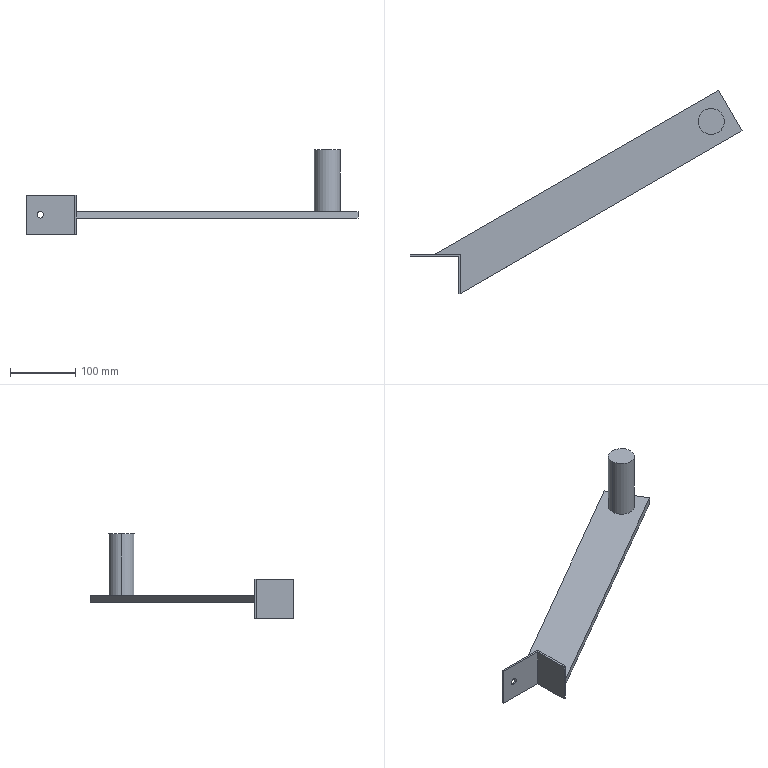Part | STEP file | 1 solid | 19 faces | box 510.013 x 312.321 x 130 mm | volume 492742 mm3 | plane 15 | cylinder 4 | commonest cylinder face diameters 10 x2 40 x2
STEP:
#1=CARTESIAN_POINT('',(0.,0.,0.));
#2=DIRECTION('',(0.,0.,1.));
#3=DIRECTION('',(1.,0.,0.));
#4=AXIS2_PLACEMENT_3D('',#1,#2,#3);
#5=CARTESIAN_POINT('',(-3.745,29.61,-5.));
#6=VERTEX_POINT('',#5);
#7=CARTESIAN_POINT('',(-3.745,26.61,-5.));
#8=VERTEX_POINT('',#7);
#9=CARTESIAN_POINT('',(-3.745,29.61,-5.));
#10=DIRECTION('',(0.,-1.,0.));
#11=VECTOR('',#10,1.);
#12=LINE('',#9,#11);
#13=CARTESIAN_POINT('',(-3.745,29.61,0.));
#14=DIRECTION('',(0.,-1.,0.));
#15=DIRECTION('',(0.,0.,-1.));
#16=AXIS2_PLACEMENT_3D('',#13,#14,#15);
#17=CYLINDRICAL_SURFACE('',#16,5.);
#18=CARTESIAN_POINT('',(6.283,0.));
#19=DIRECTION('',(0.,1.));
#20=VECTOR('',#19,1.);
#21=LINE('',#18,#20);
#22=(GEOMETRIC_REPRESENTATION_CONTEXT(2)PARAMETRIC_REPRESENTATION_CONTEXT()REPRESENTATION_CONTEXT('',''));
#23=DEFINITIONAL_REPRESENTATION('',(#21),#22);
#24=PCURVE('',#17,#23);
#25=CARTESIAN_POINT('',(-3.745,29.61,0.));
#26=DIRECTION('',(0.,-1.,0.));
#27=DIRECTION('',(0.,0.,-1.));
#28=AXIS2_PLACEMENT_3D('',#25,#26,#27);
#29=CYLINDRICAL_SURFACE('',#28,5.);
#30=CARTESIAN_POINT('',(0.,0.));
#31=DIRECTION('',(0.,1.));
#32=VECTOR('',#31,1.);
#33=LINE('',#30,#32);
#34=(GEOMETRIC_REPRESENTATION_CONTEXT(2)PARAMETRIC_REPRESENTATION_CONTEXT()REPRESENTATION_CONTEXT('',''));
#35=DEFINITIONAL_REPRESENTATION('',(#33),#34);
#36=PCURVE('',#29,#35);
#37=SURFACE_CURVE('',#12,(#24,#36),.PCURVE_S1.);
#38=EDGE_CURVE('',#6,#8,#37,.T.);
#39=ORIENTED_EDGE('',*,*,#38,.T.);
#40=CARTESIAN_POINT('',(-3.745,26.61,5.));
#41=VERTEX_POINT('',#40);
#42=CARTESIAN_POINT('',(-3.745,26.61,0.));
#43=DIRECTION('',(0.,1.,0.));
#44=DIRECTION('',(0.,0.,-1.));
#45=AXIS2_PLACEMENT_3D('',#42,#43,#44);
#46=CIRCLE('',#45,5.);
#47=CARTESIAN_POINT('',(6.283,3.));
#48=DIRECTION('',(-1.,0.));
#49=VECTOR('',#48,1.);
#50=LINE('',#47,#49);
#51=(GEOMETRIC_REPRESENTATION_CONTEXT(2)PARAMETRIC_REPRESENTATION_CONTEXT()REPRESENTATION_CONTEXT('',''));
#52=DEFINITIONAL_REPRESENTATION('',(#50),#51);
#53=PCURVE('',#17,#52);
#54=CARTESIAN_POINT('',(-25.745,26.61,0.));
#55=DIRECTION('',(0.,-1.,0.));
#56=DIRECTION('',(1.,0.,0.));
#57=AXIS2_PLACEMENT_3D('',#54,#55,#56);
#58=PLANE('',#57);
#59=CARTESIAN_POINT('',(22.,-5.));
#60=CARTESIAN_POINT('',(13.34,-5.));
#61=CARTESIAN_POINT('',(17.67,2.5));
#62=CARTESIAN_POINT('',(22.,10.));
#63=CARTESIAN_POINT('',(26.33,2.5));
#64=CARTESIAN_POINT('',(30.66,-5.));
#65=CARTESIAN_POINT('',(22.,-5.));
#66=(BOUNDED_CURVE()B_SPLINE_CURVE(2,(#59,#60,#61,#62,#63,#64,#65),.UNSPECIFIED.,.T.,.F.)B_SPLINE_CURVE_WITH_KNOTS((1,2,2,2,2,1),(-2.094,0.,2.094,4.189,6.283,8.378),.UNSPECIFIED.)CURVE()GEOMETRIC_REPRESENTATION_ITEM()RATIONAL_B_SPLINE_CURVE((1.,0.5,1.,0.5,1.,0.5,1.))REPRESENTATION_ITEM(''));
#67=(GEOMETRIC_REPRESENTATION_CONTEXT(2)PARAMETRIC_REPRESENTATION_CONTEXT()REPRESENTATION_CONTEXT('',''));
#68=DEFINITIONAL_REPRESENTATION('',(#66),#67);
#69=PCURVE('',#58,#68);
#70=SURFACE_CURVE('',#46,(#53,#69),.PCURVE_S1.);
#71=EDGE_CURVE('',#8,#41,#70,.T.);
#72=ORIENTED_EDGE('',*,*,#71,.T.);
#73=CARTESIAN_POINT('',(-3.745,29.61,5.));
#74=VERTEX_POINT('',#73);
#75=CARTESIAN_POINT('',(-3.745,29.61,5.));
#76=DIRECTION('',(0.,-1.,0.));
#77=VECTOR('',#76,1.);
#78=LINE('',#75,#77);
#79=CARTESIAN_POINT('',(3.142,0.));
#80=DIRECTION('',(0.,1.));
#81=VECTOR('',#80,1.);
#82=LINE('',#79,#81);
#83=(GEOMETRIC_REPRESENTATION_CONTEXT(2)PARAMETRIC_REPRESENTATION_CONTEXT()REPRESENTATION_CONTEXT('',''));
#84=DEFINITIONAL_REPRESENTATION('',(#82),#83);
#85=PCURVE('',#17,#84);
#86=CARTESIAN_POINT('',(3.142,0.));
#87=DIRECTION('',(0.,1.));
#88=VECTOR('',#87,1.);
#89=LINE('',#86,#88);
#90=(GEOMETRIC_REPRESENTATION_CONTEXT(2)PARAMETRIC_REPRESENTATION_CONTEXT()REPRESENTATION_CONTEXT('',''));
#91=DEFINITIONAL_REPRESENTATION('',(#89),#90);
#92=PCURVE('',#29,#91);
#93=SURFACE_CURVE('',#78,(#85,#92),.PCURVE_S1.);
#94=EDGE_CURVE('',#74,#41,#93,.T.);
#95=ORIENTED_EDGE('',*,*,#94,.F.);
#96=CARTESIAN_POINT('',(-3.745,29.61,0.));
#97=DIRECTION('',(0.,-1.,0.));
#98=DIRECTION('',(0.,0.,-1.));
#99=AXIS2_PLACEMENT_3D('',#96,#97,#98);
#100=CIRCLE('',#99,5.);
#101=CARTESIAN_POINT('',(0.,0.));
#102=DIRECTION('',(1.,0.));
#103=VECTOR('',#102,1.);
#104=LINE('',#101,#103);
#105=(GEOMETRIC_REPRESENTATION_CONTEXT(2)PARAMETRIC_REPRESENTATION_CONTEXT()REPRESENTATION_CONTEXT('',''));
#106=DEFINITIONAL_REPRESENTATION('',(#104),#105);
#107=PCURVE('',#17,#106);
#108=CARTESIAN_POINT('',(51.255,29.61,0.));
#109=DIRECTION('',(0.,1.,0.));
#110=DIRECTION('',(0.,0.,1.));
#111=AXIS2_PLACEMENT_3D('',#108,#109,#110);
#112=PLANE('',#111);
#113=CARTESIAN_POINT('',(-5.,-55.));
#114=CARTESIAN_POINT('',(-5.,-46.34));
#115=CARTESIAN_POINT('',(2.5,-50.67));
#116=CARTESIAN_POINT('',(10.,-55.));
#117=CARTESIAN_POINT('',(2.5,-59.33));
#118=CARTESIAN_POINT('',(-5.,-63.66));
#119=CARTESIAN_POINT('',(-5.,-55.));
#120=(BOUNDED_CURVE()B_SPLINE_CURVE(2,(#113,#114,#115,#116,#117,#118,#119),.UNSPECIFIED.,.T.,.F.)B_SPLINE_CURVE_WITH_KNOTS((1,2,2,2,2,1),(-2.094,0.,2.094,4.189,6.283,8.378),.UNSPECIFIED.)CURVE()GEOMETRIC_REPRESENTATION_ITEM()RATIONAL_B_SPLINE_CURVE((1.,0.5,1.,0.5,1.,0.5,1.))REPRESENTATION_ITEM(''));
#121=(GEOMETRIC_REPRESENTATION_CONTEXT(2)PARAMETRIC_REPRESENTATION_CONTEXT()REPRESENTATION_CONTEXT('',''));
#122=DEFINITIONAL_REPRESENTATION('',(#120),#121);
#123=PCURVE('',#112,#122);
#124=SURFACE_CURVE('',#100,(#107,#123),.PCURVE_S1.);
#125=EDGE_CURVE('',#74,#6,#124,.T.);
#126=ORIENTED_EDGE('',*,*,#125,.T.);
#127=EDGE_LOOP('',(#39,#72,#95,#126));
#128=FACE_BOUND('',#127,.F.);
#129=ADVANCED_FACE('',(#128),#17,.F.);
#130=CARTESIAN_POINT('',(417.097,233.973,5.));
#131=VERTEX_POINT('',#130);
#132=CARTESIAN_POINT('',(457.097,233.973,5.));
#133=VERTEX_POINT('',#132);
#134=CARTESIAN_POINT('',(437.097,233.973,5.));
#135=DIRECTION('',(0.,0.,-1.));
#136=DIRECTION('',(1.,0.,0.));
#137=AXIS2_PLACEMENT_3D('',#134,#135,#136);
#138=CIRCLE('',#137,20.);
#139=CARTESIAN_POINT('',(437.097,233.973,5.));
#140=DIRECTION('',(0.,0.,1.));
#141=DIRECTION('',(1.,0.,0.));
#142=AXIS2_PLACEMENT_3D('',#139,#140,#141);
#143=CYLINDRICAL_SURFACE('',#142,20.);
#144=CARTESIAN_POINT('',(6.283,0.));
#145=DIRECTION('',(-1.,0.));
#146=VECTOR('',#145,1.);
#147=LINE('',#144,#146);
#148=(GEOMETRIC_REPRESENTATION_CONTEXT(2)PARAMETRIC_REPRESENTATION_CONTEXT()REPRESENTATION_CONTEXT('',''));
#149=DEFINITIONAL_REPRESENTATION('',(#147),#148);
#150=PCURVE('',#143,#149);
#151=CARTESIAN_POINT('',(244.528,123.338,5.));
#152=DIRECTION('',(0.,0.,1.));
#153=DIRECTION('',(1.,0.,0.));
#154=AXIS2_PLACEMENT_3D('',#151,#152,#153);
#155=PLANE('',#154);
#156=CARTESIAN_POINT('',(212.569,110.635));
#157=CARTESIAN_POINT('',(212.569,75.994));
#158=CARTESIAN_POINT('',(182.569,93.314));
#159=CARTESIAN_POINT('',(152.569,110.635));
#160=CARTESIAN_POINT('',(182.569,127.955));
#161=CARTESIAN_POINT('',(212.569,145.276));
#162=CARTESIAN_POINT('',(212.569,110.635));
#163=(BOUNDED_CURVE()B_SPLINE_CURVE(2,(#156,#157,#158,#159,#160,#161,#162),.UNSPECIFIED.,.T.,.F.)B_SPLINE_CURVE_WITH_KNOTS((1,2,2,2,2,1),(-2.094,0.,2.094,4.189,6.283,8.378),.UNSPECIFIED.)CURVE()GEOMETRIC_REPRESENTATION_ITEM()RATIONAL_B_SPLINE_CURVE((1.,0.5,1.,0.5,1.,0.5,1.))REPRESENTATION_ITEM(''));
#164=(GEOMETRIC_REPRESENTATION_CONTEXT(2)PARAMETRIC_REPRESENTATION_CONTEXT()REPRESENTATION_CONTEXT('',''));
#165=DEFINITIONAL_REPRESENTATION('',(#163),#164);
#166=PCURVE('',#155,#165);
#167=SURFACE_CURVE('',#138,(#150,#166),.PCURVE_S1.);
#168=EDGE_CURVE('',#131,#133,#167,.T.);
#169=ORIENTED_EDGE('',*,*,#168,.F.);
#170=CARTESIAN_POINT('',(417.097,233.973,100.));
#171=VERTEX_POINT('',#170);
#172=CARTESIAN_POINT('',(417.097,233.973,5.));
#173=DIRECTION('',(0.,0.,1.));
#174=VECTOR('',#173,1.);
#175=LINE('',#172,#174);
#176=CARTESIAN_POINT('',(3.142,0.));
#177=DIRECTION('',(0.,1.));
#178=VECTOR('',#177,1.);
#179=LINE('',#176,#178);
#180=(GEOMETRIC_REPRESENTATION_CONTEXT(2)PARAMETRIC_REPRESENTATION_CONTEXT()REPRESENTATION_CONTEXT('',''));
#181=DEFINITIONAL_REPRESENTATION('',(#179),#180);
#182=PCURVE('',#143,#181);
#183=CARTESIAN_POINT('',(437.097,233.973,5.));
#184=DIRECTION('',(0.,0.,1.));
#185=DIRECTION('',(1.,0.,0.));
#186=AXIS2_PLACEMENT_3D('',#183,#184,#185);
#187=CYLINDRICAL_SURFACE('',#186,20.);
#188=CARTESIAN_POINT('',(3.142,0.));
#189=DIRECTION('',(0.,1.));
#190=VECTOR('',#189,1.);
#191=LINE('',#188,#190);
#192=(GEOMETRIC_REPRESENTATION_CONTEXT(2)PARAMETRIC_REPRESENTATION_CONTEXT()REPRESENTATION_CONTEXT('',''));
#193=DEFINITIONAL_REPRESENTATION('',(#191),#192);
#194=PCURVE('',#187,#193);
#195=SURFACE_CURVE('',#175,(#182,#194),.PCURVE_S1.);
#196=EDGE_CURVE('',#131,#171,#195,.T.);
#197=ORIENTED_EDGE('',*,*,#196,.T.);
#198=CARTESIAN_POINT('',(457.097,233.973,100.));
#199=VERTEX_POINT('',#198);
#200=CARTESIAN_POINT('',(437.097,233.973,100.));
#201=DIRECTION('',(0.,0.,-1.));
#202=DIRECTION('',(1.,0.,0.));
#203=AXIS2_PLACEMENT_3D('',#200,#201,#202);
#204=CIRCLE('',#203,20.);
#205=CARTESIAN_POINT('',(6.283,95.));
#206=DIRECTION('',(-1.,0.));
#207=VECTOR('',#206,1.);
#208=LINE('',#205,#207);
#209=(GEOMETRIC_REPRESENTATION_CONTEXT(2)PARAMETRIC_REPRESENTATION_CONTEXT()REPRESENTATION_CONTEXT('',''));
#210=DEFINITIONAL_REPRESENTATION('',(#208),#209);
#211=PCURVE('',#143,#210);
#212=CARTESIAN_POINT('',(437.097,233.973,100.));
#213=DIRECTION('',(0.,0.,1.));
#214=DIRECTION('',(1.,0.,0.));
#215=AXIS2_PLACEMENT_3D('',#212,#213,#214);
#216=PLANE('',#215);
#217=CARTESIAN_POINT('',(20.,0.));
#218=CARTESIAN_POINT('',(20.,-34.641));
#219=CARTESIAN_POINT('',(-10.,-17.321));
#220=CARTESIAN_POINT('',(-40.,0.));
#221=CARTESIAN_POINT('',(-10.,17.321));
#222=CARTESIAN_POINT('',(20.,34.641));
#223=CARTESIAN_POINT('',(20.,0.));
#224=(BOUNDED_CURVE()B_SPLINE_CURVE(2,(#217,#218,#219,#220,#221,#222,#223),.UNSPECIFIED.,.T.,.F.)B_SPLINE_CURVE_WITH_KNOTS((1,2,2,2,2,1),(-2.094,0.,2.094,4.189,6.283,8.378),.UNSPECIFIED.)CURVE()GEOMETRIC_REPRESENTATION_ITEM()RATIONAL_B_SPLINE_CURVE((1.,0.5,1.,0.5,1.,0.5,1.))REPRESENTATION_ITEM(''));
#225=(GEOMETRIC_REPRESENTATION_CONTEXT(2)PARAMETRIC_REPRESENTATION_CONTEXT()REPRESENTATION_CONTEXT('',''));
#226=DEFINITIONAL_REPRESENTATION('',(#224),#225);
#227=PCURVE('',#216,#226);
#228=SURFACE_CURVE('',#204,(#211,#227),.PCURVE_S1.);
#229=EDGE_CURVE('',#171,#199,#228,.T.);
#230=ORIENTED_EDGE('',*,*,#229,.T.);
#231=CARTESIAN_POINT('',(457.097,233.973,5.));
#232=DIRECTION('',(0.,0.,1.));
#233=VECTOR('',#232,1.);
#234=LINE('',#231,#233);
#235=CARTESIAN_POINT('',(0.,0.));
#236=DIRECTION('',(0.,1.));
#237=VECTOR('',#236,1.);
#238=LINE('',#235,#237);
#239=(GEOMETRIC_REPRESENTATION_CONTEXT(2)PARAMETRIC_REPRESENTATION_CONTEXT()REPRESENTATION_CONTEXT('',''));
#240=DEFINITIONAL_REPRESENTATION('',(#238),#239);
#241=PCURVE('',#143,#240);
#242=CARTESIAN_POINT('',(6.283,0.));
#243=DIRECTION('',(0.,1.));
#244=VECTOR('',#243,1.);
#245=LINE('',#242,#244);
#246=(GEOMETRIC_REPRESENTATION_CONTEXT(2)PARAMETRIC_REPRESENTATION_CONTEXT()REPRESENTATION_CONTEXT('',''));
#247=DEFINITIONAL_REPRESENTATION('',(#245),#246);
#248=PCURVE('',#187,#247);
#249=SURFACE_CURVE('',#234,(#241,#248),.PCURVE_S1.);
#250=EDGE_CURVE('',#133,#199,#249,.T.);
#251=ORIENTED_EDGE('',*,*,#250,.F.);
#252=EDGE_LOOP('',(#169,#197,#230,#251));
#253=FACE_BOUND('',#252,.T.);
#254=ADVANCED_FACE('',(#253),#143,.T.);
#255=CARTESIAN_POINT('',(11.255,29.61,-5.));
#256=VERTEX_POINT('',#255);
#257=CARTESIAN_POINT('',(448.287,281.931,-5.));
#258=VERTEX_POINT('',#257);
#259=CARTESIAN_POINT('',(11.255,29.61,-5.));
#260=DIRECTION('',(0.866,0.5,0.));
#261=VECTOR('',#260,1.);
#262=LINE('',#259,#261);
#263=CARTESIAN_POINT('',(244.528,123.338,-5.));
#264=DIRECTION('',(0.,0.,-1.));
#265=DIRECTION('',(-1.,0.,0.));
#266=AXIS2_PLACEMENT_3D('',#263,#264,#265);
#267=PLANE('',#266);
#268=CARTESIAN_POINT('',(233.273,-93.728));
#269=DIRECTION('',(-0.866,0.5));
#270=VECTOR('',#269,1.);
#271=LINE('',#268,#270);
#272=(GEOMETRIC_REPRESENTATION_CONTEXT(2)PARAMETRIC_REPRESENTATION_CONTEXT()REPRESENTATION_CONTEXT('',''));
#273=DEFINITIONAL_REPRESENTATION('',(#271),#272);
#274=PCURVE('',#267,#273);
#275=CARTESIAN_POINT('',(448.287,281.931,0.));
#276=DIRECTION('',(-0.5,0.866,0.));
#277=DIRECTION('',(-0.866,-0.5,0.));
#278=AXIS2_PLACEMENT_3D('',#275,#276,#277);
#279=PLANE('',#278);
#280=CARTESIAN_POINT('',(504.641,-5.));
#281=DIRECTION('',(-1.,0.));
#282=VECTOR('',#281,1.);
#283=LINE('',#280,#282);
#284=(GEOMETRIC_REPRESENTATION_CONTEXT(2)PARAMETRIC_REPRESENTATION_CONTEXT()REPRESENTATION_CONTEXT('',''));
#285=DEFINITIONAL_REPRESENTATION('',(#283),#284);
#286=PCURVE('',#279,#285);
#287=SURFACE_CURVE('',#262,(#274,#286),.PCURVE_S1.);
#288=EDGE_CURVE('',#256,#258,#287,.T.);
#289=ORIENTED_EDGE('',*,*,#288,.T.);
#290=CARTESIAN_POINT('',(484.268,219.61,-5.));
#291=VERTEX_POINT('',#290);
#292=CARTESIAN_POINT('',(448.287,281.931,-5.));
#293=DIRECTION('',(0.5,-0.866,0.));
#294=VECTOR('',#293,1.);
#295=LINE('',#292,#294);
#296=CARTESIAN_POINT('',(-203.759,158.592));
#297=DIRECTION('',(-0.5,-0.866));
#298=VECTOR('',#297,1.);
#299=LINE('',#296,#298);
#300=(GEOMETRIC_REPRESENTATION_CONTEXT(2)PARAMETRIC_REPRESENTATION_CONTEXT()REPRESENTATION_CONTEXT('',''));
#301=DEFINITIONAL_REPRESENTATION('',(#299),#300);
#302=PCURVE('',#267,#301);
#303=CARTESIAN_POINT('',(484.268,219.61,0.));
#304=DIRECTION('',(0.866,0.5,0.));
#305=DIRECTION('',(-0.5,0.866,0.));
#306=AXIS2_PLACEMENT_3D('',#303,#304,#305);
#307=PLANE('',#306);
#308=CARTESIAN_POINT('',(71.962,-5.));
#309=DIRECTION('',(-1.,0.));
#310=VECTOR('',#309,1.);
#311=LINE('',#308,#310);
#312=(GEOMETRIC_REPRESENTATION_CONTEXT(2)PARAMETRIC_REPRESENTATION_CONTEXT()REPRESENTATION_CONTEXT('',''));
#313=DEFINITIONAL_REPRESENTATION('',(#311),#312);
#314=PCURVE('',#307,#313);
#315=SURFACE_CURVE('',#295,(#302,#314),.PCURVE_S1.);
#316=EDGE_CURVE('',#258,#291,#315,.T.);
#317=ORIENTED_EDGE('',*,*,#316,.T.);
#318=CARTESIAN_POINT('',(51.255,-30.39,-5.));
#319=VERTEX_POINT('',#318);
#320=CARTESIAN_POINT('',(484.268,219.61,-5.));
#321=DIRECTION('',(-0.866,-0.5,0.));
#322=VECTOR('',#321,1.);
#323=LINE('',#320,#322);
#324=CARTESIAN_POINT('',(-239.74,96.272));
#325=DIRECTION('',(0.866,-0.5));
#326=VECTOR('',#325,1.);
#327=LINE('',#324,#326);
#328=(GEOMETRIC_REPRESENTATION_CONTEXT(2)PARAMETRIC_REPRESENTATION_CONTEXT()REPRESENTATION_CONTEXT('',''));
#329=DEFINITIONAL_REPRESENTATION('',(#327),#328);
#330=PCURVE('',#267,#329);
#331=CARTESIAN_POINT('',(51.255,-30.39,0.));
#332=DIRECTION('',(0.5,-0.866,0.));
#333=DIRECTION('',(0.866,0.5,0.));
#334=AXIS2_PLACEMENT_3D('',#331,#332,#333);
#335=PLANE('',#334);
#336=CARTESIAN_POINT('',(500.,-5.));
#337=DIRECTION('',(-1.,0.));
#338=VECTOR('',#337,1.);
#339=LINE('',#336,#338);
#340=(GEOMETRIC_REPRESENTATION_CONTEXT(2)PARAMETRIC_REPRESENTATION_CONTEXT()REPRESENTATION_CONTEXT('',''));
#341=DEFINITIONAL_REPRESENTATION('',(#339),#340);
#342=PCURVE('',#335,#341);
#343=SURFACE_CURVE('',#323,(#330,#342),.PCURVE_S1.);
#344=EDGE_CURVE('',#291,#319,#343,.T.);
#345=ORIENTED_EDGE('',*,*,#344,.T.);
#346=CARTESIAN_POINT('',(51.255,29.61,-5.));
#347=VERTEX_POINT('',#346);
#348=CARTESIAN_POINT('',(51.255,123.338,-5.));
#349=DIRECTION('',(0.,1.,0.));
#350=VECTOR('',#349,1.);
#351=LINE('',#348,#350);
#352=CARTESIAN_POINT('',(193.273,0.));
#353=DIRECTION('',(0.,1.));
#354=VECTOR('',#353,1.);
#355=LINE('',#352,#354);
#356=(GEOMETRIC_REPRESENTATION_CONTEXT(2)PARAMETRIC_REPRESENTATION_CONTEXT()REPRESENTATION_CONTEXT('',''));
#357=DEFINITIONAL_REPRESENTATION('',(#355),#356);
#358=PCURVE('',#267,#357);
#359=CARTESIAN_POINT('',(51.255,-30.39,0.));
#360=DIRECTION('',(1.,0.,0.));
#361=DIRECTION('',(0.,0.,-1.));
#362=AXIS2_PLACEMENT_3D('',#359,#360,#361);
#363=PLANE('',#362);
#364=CARTESIAN_POINT('',(5.,153.728));
#365=DIRECTION('',(0.,1.));
#366=VECTOR('',#365,1.);
#367=LINE('',#364,#366);
#368=(GEOMETRIC_REPRESENTATION_CONTEXT(2)PARAMETRIC_REPRESENTATION_CONTEXT()REPRESENTATION_CONTEXT('',''));
#369=DEFINITIONAL_REPRESENTATION('',(#367),#368);
#370=PCURVE('',#363,#369);
#371=SURFACE_CURVE('',#351,(#358,#370),.PCURVE_S1.);
#372=EDGE_CURVE('',#319,#347,#371,.T.);
#373=ORIENTED_EDGE('',*,*,#372,.T.);
#374=CARTESIAN_POINT('',(244.528,29.61,-5.));
#375=DIRECTION('',(-1.,0.,0.));
#376=VECTOR('',#375,1.);
#377=LINE('',#374,#376);
#378=CARTESIAN_POINT('',(0.,-93.728));
#379=DIRECTION('',(1.,0.));
#380=VECTOR('',#379,1.);
#381=LINE('',#378,#380);
#382=(GEOMETRIC_REPRESENTATION_CONTEXT(2)PARAMETRIC_REPRESENTATION_CONTEXT()REPRESENTATION_CONTEXT('',''));
#383=DEFINITIONAL_REPRESENTATION('',(#381),#382);
#384=PCURVE('',#267,#383);
#385=CARTESIAN_POINT('',(-5.,193.273));
#386=DIRECTION('',(0.,-1.));
#387=VECTOR('',#386,1.);
#388=LINE('',#385,#387);
#389=(GEOMETRIC_REPRESENTATION_CONTEXT(2)PARAMETRIC_REPRESENTATION_CONTEXT()REPRESENTATION_CONTEXT('',''));
#390=DEFINITIONAL_REPRESENTATION('',(#388),#389);
#391=PCURVE('',#112,#390);
#392=SURFACE_CURVE('',#377,(#384,#391),.PCURVE_S1.);
#393=EDGE_CURVE('',#347,#256,#392,.T.);
#394=ORIENTED_EDGE('',*,*,#393,.T.);
#395=EDGE_LOOP('',(#289,#317,#345,#373,#394));
#396=FACE_BOUND('',#395,.T.);
#397=ADVANCED_FACE('',(#396),#267,.T.);
#398=CARTESIAN_POINT('',(484.268,219.61,5.));
#399=VERTEX_POINT('',#398);
#400=CARTESIAN_POINT('',(484.268,219.61,0.));
#401=DIRECTION('',(0.,0.,-1.));
#402=VECTOR('',#401,1.);
#403=LINE('',#400,#402);
#404=CARTESIAN_POINT('',(0.,0.));
#405=DIRECTION('',(0.,-1.));
#406=VECTOR('',#405,1.);
#407=LINE('',#404,#406);
#408=(GEOMETRIC_REPRESENTATION_CONTEXT(2)PARAMETRIC_REPRESENTATION_CONTEXT()REPRESENTATION_CONTEXT('',''));
#409=DEFINITIONAL_REPRESENTATION('',(#407),#408);
#410=PCURVE('',#307,#409);
#411=CARTESIAN_POINT('',(500.,0.));
#412=DIRECTION('',(0.,-1.));
#413=VECTOR('',#412,1.);
#414=LINE('',#411,#413);
#415=(GEOMETRIC_REPRESENTATION_CONTEXT(2)PARAMETRIC_REPRESENTATION_CONTEXT()REPRESENTATION_CONTEXT('',''));
#416=DEFINITIONAL_REPRESENTATION('',(#414),#415);
#417=PCURVE('',#335,#416);
#418=SURFACE_CURVE('',#403,(#410,#417),.PCURVE_S1.);
#419=EDGE_CURVE('',#399,#291,#418,.T.);
#420=ORIENTED_EDGE('',*,*,#419,.T.);
#421=ORIENTED_EDGE('',*,*,#316,.F.);
#422=CARTESIAN_POINT('',(448.287,281.931,5.));
#423=VERTEX_POINT('',#422);
#424=CARTESIAN_POINT('',(448.287,281.931,0.));
#425=DIRECTION('',(0.,0.,1.));
#426=VECTOR('',#425,1.);
#427=LINE('',#424,#426);
#428=CARTESIAN_POINT('',(71.962,0.));
#429=DIRECTION('',(0.,1.));
#430=VECTOR('',#429,1.);
#431=LINE('',#428,#430);
#432=(GEOMETRIC_REPRESENTATION_CONTEXT(2)PARAMETRIC_REPRESENTATION_CONTEXT()REPRESENTATION_CONTEXT('',''));
#433=DEFINITIONAL_REPRESENTATION('',(#431),#432);
#434=PCURVE('',#307,#433);
#435=CARTESIAN_POINT('',(0.,0.));
#436=DIRECTION('',(0.,1.));
#437=VECTOR('',#436,1.);
#438=LINE('',#435,#437);
#439=(GEOMETRIC_REPRESENTATION_CONTEXT(2)PARAMETRIC_REPRESENTATION_CONTEXT()REPRESENTATION_CONTEXT('',''));
#440=DEFINITIONAL_REPRESENTATION('',(#438),#439);
#441=PCURVE('',#279,#440);
#442=SURFACE_CURVE('',#427,(#434,#441),.PCURVE_S1.);
#443=EDGE_CURVE('',#258,#423,#442,.T.);
#444=ORIENTED_EDGE('',*,*,#443,.T.);
#445=CARTESIAN_POINT('',(484.268,219.61,5.));
#446=DIRECTION('',(0.5,-0.866,0.));
#447=VECTOR('',#446,1.);
#448=LINE('',#445,#447);
#449=CARTESIAN_POINT('',(0.,5.));
#450=DIRECTION('',(-1.,0.));
#451=VECTOR('',#450,1.);
#452=LINE('',#449,#451);
#453=(GEOMETRIC_REPRESENTATION_CONTEXT(2)PARAMETRIC_REPRESENTATION_CONTEXT()REPRESENTATION_CONTEXT('',''));
#454=DEFINITIONAL_REPRESENTATION('',(#452),#453);
#455=PCURVE('',#307,#454);
#456=CARTESIAN_POINT('',(239.74,96.272));
#457=DIRECTION('',(0.5,-0.866));
#458=VECTOR('',#457,1.);
#459=LINE('',#456,#458);
#460=(GEOMETRIC_REPRESENTATION_CONTEXT(2)PARAMETRIC_REPRESENTATION_CONTEXT()REPRESENTATION_CONTEXT('',''));
#461=DEFINITIONAL_REPRESENTATION('',(#459),#460);
#462=PCURVE('',#155,#461);
#463=SURFACE_CURVE('',#448,(#455,#462),.PCURVE_S1.);
#464=EDGE_CURVE('',#423,#399,#463,.T.);
#465=ORIENTED_EDGE('',*,*,#464,.T.);
#466=EDGE_LOOP('',(#420,#421,#444,#465));
#467=FACE_BOUND('',#466,.T.);
#468=ADVANCED_FACE('',(#467),#307,.T.);
#469=ORIENTED_EDGE('',*,*,#443,.F.);
#470=ORIENTED_EDGE('',*,*,#288,.F.);
#471=CARTESIAN_POINT('',(11.255,29.61,5.));
#472=VERTEX_POINT('',#471);
#473=CARTESIAN_POINT('',(11.255,29.61,0.));
#474=DIRECTION('',(0.,0.,1.));
#475=VECTOR('',#474,1.);
#476=LINE('',#473,#475);
#477=CARTESIAN_POINT('',(504.641,0.));
#478=DIRECTION('',(0.,1.));
#479=VECTOR('',#478,1.);
#480=LINE('',#477,#479);
#481=(GEOMETRIC_REPRESENTATION_CONTEXT(2)PARAMETRIC_REPRESENTATION_CONTEXT()REPRESENTATION_CONTEXT('',''));
#482=DEFINITIONAL_REPRESENTATION('',(#480),#481);
#483=PCURVE('',#279,#482);
#484=CARTESIAN_POINT('',(0.,-40.));
#485=DIRECTION('',(1.,0.));
#486=VECTOR('',#485,1.);
#487=LINE('',#484,#486);
#488=(GEOMETRIC_REPRESENTATION_CONTEXT(2)PARAMETRIC_REPRESENTATION_CONTEXT()REPRESENTATION_CONTEXT('',''));
#489=DEFINITIONAL_REPRESENTATION('',(#487),#488);
#490=PCURVE('',#112,#489);
#491=SURFACE_CURVE('',#476,(#483,#490),.PCURVE_S1.);
#492=EDGE_CURVE('',#256,#472,#491,.T.);
#493=ORIENTED_EDGE('',*,*,#492,.T.);
#494=CARTESIAN_POINT('',(448.287,281.931,5.));
#495=DIRECTION('',(0.866,0.5,0.));
#496=VECTOR('',#495,1.);
#497=LINE('',#494,#496);
#498=CARTESIAN_POINT('',(0.,5.));
#499=DIRECTION('',(-1.,0.));
#500=VECTOR('',#499,1.);
#501=LINE('',#498,#500);
#502=(GEOMETRIC_REPRESENTATION_CONTEXT(2)PARAMETRIC_REPRESENTATION_CONTEXT()REPRESENTATION_CONTEXT('',''));
#503=DEFINITIONAL_REPRESENTATION('',(#501),#502);
#504=PCURVE('',#279,#503);
#505=CARTESIAN_POINT('',(203.759,158.592));
#506=DIRECTION('',(0.866,0.5));
#507=VECTOR('',#506,1.);
#508=LINE('',#505,#507);
#509=(GEOMETRIC_REPRESENTATION_CONTEXT(2)PARAMETRIC_REPRESENTATION_CONTEXT()REPRESENTATION_CONTEXT('',''));
#510=DEFINITIONAL_REPRESENTATION('',(#508),#509);
#511=PCURVE('',#155,#510);
#512=SURFACE_CURVE('',#497,(#504,#511),.PCURVE_S1.);
#513=EDGE_CURVE('',#472,#423,#512,.T.);
#514=ORIENTED_EDGE('',*,*,#513,.T.);
#515=EDGE_LOOP('',(#469,#470,#493,#514));
#516=FACE_BOUND('',#515,.T.);
#517=ADVANCED_FACE('',(#516),#279,.T.);
#518=CARTESIAN_POINT('',(-25.745,29.61,30.));
#519=VERTEX_POINT('',#518);
#520=CARTESIAN_POINT('',(51.255,29.61,30.));
#521=VERTEX_POINT('',#520);
#522=CARTESIAN_POINT('',(51.255,29.61,30.));
#523=DIRECTION('',(1.,0.,0.));
#524=VECTOR('',#523,1.);
#525=LINE('',#522,#524);
#526=CARTESIAN_POINT('',(30.,0.));
#527=DIRECTION('',(0.,1.));
#528=VECTOR('',#527,1.);
#529=LINE('',#526,#528);
#530=(GEOMETRIC_REPRESENTATION_CONTEXT(2)PARAMETRIC_REPRESENTATION_CONTEXT()REPRESENTATION_CONTEXT('',''));
#531=DEFINITIONAL_REPRESENTATION('',(#529),#530);
#532=PCURVE('',#112,#531);
#533=CARTESIAN_POINT('',(28.15,15.005,30.));
#534=DIRECTION('',(0.,0.,1.));
#535=DIRECTION('',(1.,0.,0.));
#536=AXIS2_PLACEMENT_3D('',#533,#534,#535);
#537=PLANE('',#536);
#538=CARTESIAN_POINT('',(23.106,14.606));
#539=DIRECTION('',(1.,0.));
#540=VECTOR('',#539,1.);
#541=LINE('',#538,#540);
#542=(GEOMETRIC_REPRESENTATION_CONTEXT(2)PARAMETRIC_REPRESENTATION_CONTEXT()REPRESENTATION_CONTEXT('',''));
#543=DEFINITIONAL_REPRESENTATION('',(#541),#542);
#544=PCURVE('',#537,#543);
#545=SURFACE_CURVE('',#525,(#532,#544),.PCURVE_S1.);
#546=EDGE_CURVE('',#519,#521,#545,.T.);
#547=ORIENTED_EDGE('',*,*,#546,.T.);
#548=CARTESIAN_POINT('',(51.255,29.61,5.));
#549=VERTEX_POINT('',#548);
#550=CARTESIAN_POINT('',(51.255,29.61,0.));
#551=DIRECTION('',(0.,0.,-1.));
#552=VECTOR('',#551,1.);
#553=LINE('',#550,#552);
#554=CARTESIAN_POINT('',(0.,0.));
#555=DIRECTION('',(-1.,0.));
#556=VECTOR('',#555,1.);
#557=LINE('',#554,#556);
#558=(GEOMETRIC_REPRESENTATION_CONTEXT(2)PARAMETRIC_REPRESENTATION_CONTEXT()REPRESENTATION_CONTEXT('',''));
#559=DEFINITIONAL_REPRESENTATION('',(#557),#558);
#560=PCURVE('',#112,#559);
#561=CARTESIAN_POINT('',(51.255,-30.39,0.));
#562=DIRECTION('',(1.,0.,0.));
#563=DIRECTION('',(0.,0.,-1.));
#564=AXIS2_PLACEMENT_3D('',#561,#562,#563);
#565=PLANE('',#564);
#566=CARTESIAN_POINT('',(0.,60.));
#567=DIRECTION('',(1.,0.));
#568=VECTOR('',#567,1.);
#569=LINE('',#566,#568);
#570=(GEOMETRIC_REPRESENTATION_CONTEXT(2)PARAMETRIC_REPRESENTATION_CONTEXT()REPRESENTATION_CONTEXT('',''));
#571=DEFINITIONAL_REPRESENTATION('',(#569),#570);
#572=PCURVE('',#565,#571);
#573=SURFACE_CURVE('',#553,(#560,#572),.PCURVE_S1.);
#574=EDGE_CURVE('',#521,#549,#573,.T.);
#575=ORIENTED_EDGE('',*,*,#574,.T.);
#576=CARTESIAN_POINT('',(51.255,29.61,5.));
#577=DIRECTION('',(-1.,0.,0.));
#578=VECTOR('',#577,1.);
#579=LINE('',#576,#578);
#580=CARTESIAN_POINT('',(5.,0.));
#581=DIRECTION('',(0.,-1.));
#582=VECTOR('',#581,1.);
#583=LINE('',#580,#582);
#584=(GEOMETRIC_REPRESENTATION_CONTEXT(2)PARAMETRIC_REPRESENTATION_CONTEXT()REPRESENTATION_CONTEXT('',''));
#585=DEFINITIONAL_REPRESENTATION('',(#583),#584);
#586=PCURVE('',#112,#585);
#587=CARTESIAN_POINT('',(-193.273,-93.728));
#588=DIRECTION('',(-1.,0.));
#589=VECTOR('',#588,1.);
#590=LINE('',#587,#589);
#591=(GEOMETRIC_REPRESENTATION_CONTEXT(2)PARAMETRIC_REPRESENTATION_CONTEXT()REPRESENTATION_CONTEXT('',''));
#592=DEFINITIONAL_REPRESENTATION('',(#590),#591);
#593=PCURVE('',#155,#592);
#594=SURFACE_CURVE('',#579,(#586,#593),.PCURVE_S1.);
#595=EDGE_CURVE('',#549,#472,#594,.T.);
#596=ORIENTED_EDGE('',*,*,#595,.T.);
#597=ORIENTED_EDGE('',*,*,#492,.F.);
#598=ORIENTED_EDGE('',*,*,#393,.F.);
#599=CARTESIAN_POINT('',(51.255,29.61,-30.));
#600=VERTEX_POINT('',#599);
#601=CARTESIAN_POINT('',(51.255,29.61,0.));
#602=DIRECTION('',(0.,0.,-1.));
#603=VECTOR('',#602,1.);
#604=LINE('',#601,#603);
#605=CARTESIAN_POINT('',(0.,0.));
#606=DIRECTION('',(-1.,0.));
#607=VECTOR('',#606,1.);
#608=LINE('',#605,#607);
#609=(GEOMETRIC_REPRESENTATION_CONTEXT(2)PARAMETRIC_REPRESENTATION_CONTEXT()REPRESENTATION_CONTEXT('',''));
#610=DEFINITIONAL_REPRESENTATION('',(#608),#609);
#611=PCURVE('',#112,#610);
#612=CARTESIAN_POINT('',(0.,60.));
#613=DIRECTION('',(1.,0.));
#614=VECTOR('',#613,1.);
#615=LINE('',#612,#614);
#616=(GEOMETRIC_REPRESENTATION_CONTEXT(2)PARAMETRIC_REPRESENTATION_CONTEXT()REPRESENTATION_CONTEXT('',''));
#617=DEFINITIONAL_REPRESENTATION('',(#615),#616);
#618=PCURVE('',#363,#617);
#619=SURFACE_CURVE('',#604,(#611,#618),.PCURVE_S1.);
#620=EDGE_CURVE('',#347,#600,#619,.T.);
#621=ORIENTED_EDGE('',*,*,#620,.T.);
#622=CARTESIAN_POINT('',(-25.745,29.61,-30.));
#623=VERTEX_POINT('',#622);
#624=CARTESIAN_POINT('',(51.255,29.61,-30.));
#625=DIRECTION('',(-1.,0.,0.));
#626=VECTOR('',#625,1.);
#627=LINE('',#624,#626);
#628=CARTESIAN_POINT('',(-30.,0.));
#629=DIRECTION('',(0.,-1.));
#630=VECTOR('',#629,1.);
#631=LINE('',#628,#630);
#632=(GEOMETRIC_REPRESENTATION_CONTEXT(2)PARAMETRIC_REPRESENTATION_CONTEXT()REPRESENTATION_CONTEXT('',''));
#633=DEFINITIONAL_REPRESENTATION('',(#631),#632);
#634=PCURVE('',#112,#633);
#635=CARTESIAN_POINT('',(28.15,15.005,-30.));
#636=DIRECTION('',(0.,0.,-1.));
#637=DIRECTION('',(-1.,0.,0.));
#638=AXIS2_PLACEMENT_3D('',#635,#636,#637);
#639=PLANE('',#638);
#640=CARTESIAN_POINT('',(-23.106,14.606));
#641=DIRECTION('',(1.,0.));
#642=VECTOR('',#641,1.);
#643=LINE('',#640,#642);
#644=(GEOMETRIC_REPRESENTATION_CONTEXT(2)PARAMETRIC_REPRESENTATION_CONTEXT()REPRESENTATION_CONTEXT('',''));
#645=DEFINITIONAL_REPRESENTATION('',(#643),#644);
#646=PCURVE('',#639,#645);
#647=SURFACE_CURVE('',#627,(#634,#646),.PCURVE_S1.);
#648=EDGE_CURVE('',#600,#623,#647,.T.);
#649=ORIENTED_EDGE('',*,*,#648,.T.);
#650=CARTESIAN_POINT('',(-25.745,29.61,0.));
#651=DIRECTION('',(0.,0.,1.));
#652=VECTOR('',#651,1.);
#653=LINE('',#650,#652);
#654=CARTESIAN_POINT('',(0.,-77.));
#655=DIRECTION('',(1.,0.));
#656=VECTOR('',#655,1.);
#657=LINE('',#654,#656);
#658=(GEOMETRIC_REPRESENTATION_CONTEXT(2)PARAMETRIC_REPRESENTATION_CONTEXT()REPRESENTATION_CONTEXT('',''));
#659=DEFINITIONAL_REPRESENTATION('',(#657),#658);
#660=PCURVE('',#112,#659);
#661=CARTESIAN_POINT('',(-25.745,29.61,0.));
#662=DIRECTION('',(-1.,0.,0.));
#663=DIRECTION('',(0.,0.,1.));
#664=AXIS2_PLACEMENT_3D('',#661,#662,#663);
#665=PLANE('',#664);
#666=CARTESIAN_POINT('',(0.,0.));
#667=DIRECTION('',(1.,0.));
#668=VECTOR('',#667,1.);
#669=LINE('',#666,#668);
#670=(GEOMETRIC_REPRESENTATION_CONTEXT(2)PARAMETRIC_REPRESENTATION_CONTEXT()REPRESENTATION_CONTEXT('',''));
#671=DEFINITIONAL_REPRESENTATION('',(#669),#670);
#672=PCURVE('',#665,#671);
#673=SURFACE_CURVE('',#653,(#660,#672),.PCURVE_S1.);
#674=EDGE_CURVE('',#623,#519,#673,.T.);
#675=ORIENTED_EDGE('',*,*,#674,.T.);
#676=EDGE_LOOP('',(#547,#575,#596,#597,#598,#621,#649,#675));
#677=FACE_BOUND('',#676,.T.);
#678=CARTESIAN_POINT('',(-3.745,29.61,0.));
#679=DIRECTION('',(0.,-1.,0.));
#680=DIRECTION('',(0.,0.,-1.));
#681=AXIS2_PLACEMENT_3D('',#678,#679,#680);
#682=CIRCLE('',#681,5.);
#683=CARTESIAN_POINT('',(-5.,-55.));
#684=CARTESIAN_POINT('',(-5.,-46.34));
#685=CARTESIAN_POINT('',(2.5,-50.67));
#686=CARTESIAN_POINT('',(10.,-55.));
#687=CARTESIAN_POINT('',(2.5,-59.33));
#688=CARTESIAN_POINT('',(-5.,-63.66));
#689=CARTESIAN_POINT('',(-5.,-55.));
#690=(BOUNDED_CURVE()B_SPLINE_CURVE(2,(#683,#684,#685,#686,#687,#688,#689),.UNSPECIFIED.,.T.,.F.)B_SPLINE_CURVE_WITH_KNOTS((1,2,2,2,2,1),(-2.094,0.,2.094,4.189,6.283,8.378),.UNSPECIFIED.)CURVE()GEOMETRIC_REPRESENTATION_ITEM()RATIONAL_B_SPLINE_CURVE((1.,0.5,1.,0.5,1.,0.5,1.))REPRESENTATION_ITEM(''));
#691=(GEOMETRIC_REPRESENTATION_CONTEXT(2)PARAMETRIC_REPRESENTATION_CONTEXT()REPRESENTATION_CONTEXT('',''));
#692=DEFINITIONAL_REPRESENTATION('',(#690),#691);
#693=PCURVE('',#112,#692);
#694=CARTESIAN_POINT('',(0.,0.));
#695=DIRECTION('',(1.,0.));
#696=VECTOR('',#695,1.);
#697=LINE('',#694,#696);
#698=(GEOMETRIC_REPRESENTATION_CONTEXT(2)PARAMETRIC_REPRESENTATION_CONTEXT()REPRESENTATION_CONTEXT('',''));
#699=DEFINITIONAL_REPRESENTATION('',(#697),#698);
#700=PCURVE('',#29,#699);
#701=SURFACE_CURVE('',#682,(#693,#700),.PCURVE_S1.);
#702=EDGE_CURVE('',#6,#74,#701,.T.);
#703=ORIENTED_EDGE('',*,*,#702,.T.);
#704=ORIENTED_EDGE('',*,*,#125,.T.);
#705=EDGE_LOOP('',(#703,#704));
#706=FACE_BOUND('',#705,.T.);
#707=ADVANCED_FACE('',(#677,#706),#112,.T.);
#708=CARTESIAN_POINT('',(51.255,-30.39,-30.));
#709=VERTEX_POINT('',#708);
#710=CARTESIAN_POINT('',(51.255,-30.39,-30.));
#711=DIRECTION('',(0.,1.,0.));
#712=VECTOR('',#711,1.);
#713=LINE('',#710,#712);
#714=CARTESIAN_POINT('',(30.,0.));
#715=DIRECTION('',(0.,1.));
#716=VECTOR('',#715,1.);
#717=LINE('',#714,#716);
#718=(GEOMETRIC_REPRESENTATION_CONTEXT(2)PARAMETRIC_REPRESENTATION_CONTEXT()REPRESENTATION_CONTEXT('',''));
#719=DEFINITIONAL_REPRESENTATION('',(#717),#718);
#720=PCURVE('',#363,#719);
#721=CARTESIAN_POINT('',(-23.106,-45.394));
#722=DIRECTION('',(0.,1.));
#723=VECTOR('',#722,1.);
#724=LINE('',#721,#723);
#725=(GEOMETRIC_REPRESENTATION_CONTEXT(2)PARAMETRIC_REPRESENTATION_CONTEXT()REPRESENTATION_CONTEXT('',''));
#726=DEFINITIONAL_REPRESENTATION('',(#724),#725);
#727=PCURVE('',#639,#726);
#728=SURFACE_CURVE('',#713,(#720,#727),.PCURVE_S1.);
#729=EDGE_CURVE('',#709,#600,#728,.T.);
#730=ORIENTED_EDGE('',*,*,#729,.T.);
#731=ORIENTED_EDGE('',*,*,#620,.F.);
#732=ORIENTED_EDGE('',*,*,#372,.F.);
#733=CARTESIAN_POINT('',(51.255,-30.39,0.));
#734=DIRECTION('',(0.,0.,-1.));
#735=VECTOR('',#734,1.);
#736=LINE('',#733,#735);
#737=CARTESIAN_POINT('',(0.,0.));
#738=DIRECTION('',(1.,0.));
#739=VECTOR('',#738,1.);
#740=LINE('',#737,#739);
#741=(GEOMETRIC_REPRESENTATION_CONTEXT(2)PARAMETRIC_REPRESENTATION_CONTEXT()REPRESENTATION_CONTEXT('',''));
#742=DEFINITIONAL_REPRESENTATION('',(#740),#741);
#743=PCURVE('',#363,#742);
#744=CARTESIAN_POINT('',(48.255,-30.39,0.));
#745=DIRECTION('',(0.,-1.,0.));
#746=DIRECTION('',(0.,0.,-1.));
#747=AXIS2_PLACEMENT_3D('',#744,#745,#746);
#748=PLANE('',#747);
#749=CARTESIAN_POINT('',(0.,3.));
#750=DIRECTION('',(1.,0.));
#751=VECTOR('',#750,1.);
#752=LINE('',#749,#751);
#753=(GEOMETRIC_REPRESENTATION_CONTEXT(2)PARAMETRIC_REPRESENTATION_CONTEXT()REPRESENTATION_CONTEXT('',''));
#754=DEFINITIONAL_REPRESENTATION('',(#752),#753);
#755=PCURVE('',#748,#754);
#756=SURFACE_CURVE('',#736,(#743,#755),.PCURVE_S1.);
#757=EDGE_CURVE('',#319,#709,#756,.T.);
#758=ORIENTED_EDGE('',*,*,#757,.T.);
#759=EDGE_LOOP('',(#730,#731,#732,#758));
#760=FACE_BOUND('',#759,.T.);
#761=ADVANCED_FACE('',(#760),#363,.T.);
#762=CARTESIAN_POINT('',(51.255,-30.39,5.));
#763=VERTEX_POINT('',#762);
#764=CARTESIAN_POINT('',(51.255,-30.39,0.));
#765=DIRECTION('',(0.,0.,-1.));
#766=VECTOR('',#765,1.);
#767=LINE('',#764,#766);
#768=CARTESIAN_POINT('',(0.,0.));
#769=DIRECTION('',(0.,-1.));
#770=VECTOR('',#769,1.);
#771=LINE('',#768,#770);
#772=(GEOMETRIC_REPRESENTATION_CONTEXT(2)PARAMETRIC_REPRESENTATION_CONTEXT()REPRESENTATION_CONTEXT('',''));
#773=DEFINITIONAL_REPRESENTATION('',(#771),#772);
#774=PCURVE('',#335,#773);
#775=CARTESIAN_POINT('',(0.,3.));
#776=DIRECTION('',(1.,0.));
#777=VECTOR('',#776,1.);
#778=LINE('',#775,#777);
#779=(GEOMETRIC_REPRESENTATION_CONTEXT(2)PARAMETRIC_REPRESENTATION_CONTEXT()REPRESENTATION_CONTEXT('',''));
#780=DEFINITIONAL_REPRESENTATION('',(#778),#779);
#781=PCURVE('',#748,#780);
#782=SURFACE_CURVE('',#767,(#774,#781),.PCURVE_S1.);
#783=EDGE_CURVE('',#763,#319,#782,.T.);
#784=ORIENTED_EDGE('',*,*,#783,.T.);
#785=ORIENTED_EDGE('',*,*,#344,.F.);
#786=ORIENTED_EDGE('',*,*,#419,.F.);
#787=CARTESIAN_POINT('',(51.255,-30.39,5.));
#788=DIRECTION('',(-0.866,-0.5,0.));
#789=VECTOR('',#788,1.);
#790=LINE('',#787,#789);
#791=CARTESIAN_POINT('',(0.,5.));
#792=DIRECTION('',(-1.,0.));
#793=VECTOR('',#792,1.);
#794=LINE('',#791,#793);
#795=(GEOMETRIC_REPRESENTATION_CONTEXT(2)PARAMETRIC_REPRESENTATION_CONTEXT()REPRESENTATION_CONTEXT('',''));
#796=DEFINITIONAL_REPRESENTATION('',(#794),#795);
#797=PCURVE('',#335,#796);
#798=CARTESIAN_POINT('',(-193.273,-153.728));
#799=DIRECTION('',(-0.866,-0.5));
#800=VECTOR('',#799,1.);
#801=LINE('',#798,#800);
#802=(GEOMETRIC_REPRESENTATION_CONTEXT(2)PARAMETRIC_REPRESENTATION_CONTEXT()REPRESENTATION_CONTEXT('',''));
#803=DEFINITIONAL_REPRESENTATION('',(#801),#802);
#804=PCURVE('',#155,#803);
#805=SURFACE_CURVE('',#790,(#797,#804),.PCURVE_S1.);
#806=EDGE_CURVE('',#399,#763,#805,.T.);
#807=ORIENTED_EDGE('',*,*,#806,.T.);
#808=EDGE_LOOP('',(#784,#785,#786,#807));
#809=FACE_BOUND('',#808,.T.);
#810=ADVANCED_FACE('',(#809),#335,.T.);
#811=ORIENTED_EDGE('',*,*,#595,.F.);
#812=CARTESIAN_POINT('',(51.255,123.338,5.));
#813=DIRECTION('',(0.,-1.,0.));
#814=VECTOR('',#813,1.);
#815=LINE('',#812,#814);
#816=CARTESIAN_POINT('',(-193.273,0.));
#817=DIRECTION('',(0.,-1.));
#818=VECTOR('',#817,1.);
#819=LINE('',#816,#818);
#820=(GEOMETRIC_REPRESENTATION_CONTEXT(2)PARAMETRIC_REPRESENTATION_CONTEXT()REPRESENTATION_CONTEXT('',''));
#821=DEFINITIONAL_REPRESENTATION('',(#819),#820);
#822=PCURVE('',#155,#821);
#823=CARTESIAN_POINT('',(-5.,153.728));
#824=DIRECTION('',(0.,-1.));
#825=VECTOR('',#824,1.);
#826=LINE('',#823,#825);
#827=(GEOMETRIC_REPRESENTATION_CONTEXT(2)PARAMETRIC_REPRESENTATION_CONTEXT()REPRESENTATION_CONTEXT('',''));
#828=DEFINITIONAL_REPRESENTATION('',(#826),#827);
#829=PCURVE('',#565,#828);
#830=SURFACE_CURVE('',#815,(#822,#829),.PCURVE_S1.);
#831=EDGE_CURVE('',#549,#763,#830,.T.);
#832=ORIENTED_EDGE('',*,*,#831,.T.);
#833=ORIENTED_EDGE('',*,*,#806,.F.);
#834=ORIENTED_EDGE('',*,*,#464,.F.);
#835=ORIENTED_EDGE('',*,*,#513,.F.);
#836=EDGE_LOOP('',(#811,#832,#833,#834,#835));
#837=FACE_BOUND('',#836,.T.);
#838=CARTESIAN_POINT('',(437.097,233.973,5.));
#839=DIRECTION('',(0.,0.,-1.));
#840=DIRECTION('',(1.,0.,0.));
#841=AXIS2_PLACEMENT_3D('',#838,#839,#840);
#842=CIRCLE('',#841,20.);
#843=CARTESIAN_POINT('',(212.569,110.635));
#844=CARTESIAN_POINT('',(212.569,75.994));
#845=CARTESIAN_POINT('',(182.569,93.314));
#846=CARTESIAN_POINT('',(152.569,110.635));
#847=CARTESIAN_POINT('',(182.569,127.955));
#848=CARTESIAN_POINT('',(212.569,145.276));
#849=CARTESIAN_POINT('',(212.569,110.635));
#850=(BOUNDED_CURVE()B_SPLINE_CURVE(2,(#843,#844,#845,#846,#847,#848,#849),.UNSPECIFIED.,.T.,.F.)B_SPLINE_CURVE_WITH_KNOTS((1,2,2,2,2,1),(-2.094,0.,2.094,4.189,6.283,8.378),.UNSPECIFIED.)CURVE()GEOMETRIC_REPRESENTATION_ITEM()RATIONAL_B_SPLINE_CURVE((1.,0.5,1.,0.5,1.,0.5,1.))REPRESENTATION_ITEM(''));
#851=(GEOMETRIC_REPRESENTATION_CONTEXT(2)PARAMETRIC_REPRESENTATION_CONTEXT()REPRESENTATION_CONTEXT('',''));
#852=DEFINITIONAL_REPRESENTATION('',(#850),#851);
#853=PCURVE('',#155,#852);
#854=CARTESIAN_POINT('',(6.283,0.));
#855=DIRECTION('',(-1.,0.));
#856=VECTOR('',#855,1.);
#857=LINE('',#854,#856);
#858=(GEOMETRIC_REPRESENTATION_CONTEXT(2)PARAMETRIC_REPRESENTATION_CONTEXT()REPRESENTATION_CONTEXT('',''));
#859=DEFINITIONAL_REPRESENTATION('',(#857),#858);
#860=PCURVE('',#187,#859);
#861=SURFACE_CURVE('',#842,(#853,#860),.PCURVE_S1.);
#862=EDGE_CURVE('',#133,#131,#861,.T.);
#863=ORIENTED_EDGE('',*,*,#862,.T.);
#864=ORIENTED_EDGE('',*,*,#168,.T.);
#865=EDGE_LOOP('',(#863,#864));
#866=FACE_BOUND('',#865,.T.);
#867=ADVANCED_FACE('',(#837,#866),#155,.T.);
#868=CARTESIAN_POINT('',(51.255,-30.39,30.));
#869=VERTEX_POINT('',#868);
#870=CARTESIAN_POINT('',(51.255,-30.39,30.));
#871=DIRECTION('',(0.,-1.,0.));
#872=VECTOR('',#871,1.);
#873=LINE('',#870,#872);
#874=CARTESIAN_POINT('',(-30.,0.));
#875=DIRECTION('',(0.,-1.));
#876=VECTOR('',#875,1.);
#877=LINE('',#874,#876);
#878=(GEOMETRIC_REPRESENTATION_CONTEXT(2)PARAMETRIC_REPRESENTATION_CONTEXT()REPRESENTATION_CONTEXT('',''));
#879=DEFINITIONAL_REPRESENTATION('',(#877),#878);
#880=PCURVE('',#565,#879);
#881=CARTESIAN_POINT('',(23.106,-45.394));
#882=DIRECTION('',(0.,-1.));
#883=VECTOR('',#882,1.);
#884=LINE('',#881,#883);
#885=(GEOMETRIC_REPRESENTATION_CONTEXT(2)PARAMETRIC_REPRESENTATION_CONTEXT()REPRESENTATION_CONTEXT('',''));
#886=DEFINITIONAL_REPRESENTATION('',(#884),#885);
#887=PCURVE('',#537,#886);
#888=SURFACE_CURVE('',#873,(#880,#887),.PCURVE_S1.);
#889=EDGE_CURVE('',#521,#869,#888,.T.);
#890=ORIENTED_EDGE('',*,*,#889,.T.);
#891=CARTESIAN_POINT('',(51.255,-30.39,0.));
#892=DIRECTION('',(0.,0.,-1.));
#893=VECTOR('',#892,1.);
#894=LINE('',#891,#893);
#895=CARTESIAN_POINT('',(0.,0.));
#896=DIRECTION('',(1.,0.));
#897=VECTOR('',#896,1.);
#898=LINE('',#895,#897);
#899=(GEOMETRIC_REPRESENTATION_CONTEXT(2)PARAMETRIC_REPRESENTATION_CONTEXT()REPRESENTATION_CONTEXT('',''));
#900=DEFINITIONAL_REPRESENTATION('',(#898),#899);
#901=PCURVE('',#565,#900);
#902=CARTESIAN_POINT('',(0.,3.));
#903=DIRECTION('',(1.,0.));
#904=VECTOR('',#903,1.);
#905=LINE('',#902,#904);
#906=(GEOMETRIC_REPRESENTATION_CONTEXT(2)PARAMETRIC_REPRESENTATION_CONTEXT()REPRESENTATION_CONTEXT('',''));
#907=DEFINITIONAL_REPRESENTATION('',(#905),#906);
#908=PCURVE('',#748,#907);
#909=SURFACE_CURVE('',#894,(#901,#908),.PCURVE_S1.);
#910=EDGE_CURVE('',#869,#763,#909,.T.);
#911=ORIENTED_EDGE('',*,*,#910,.T.);
#912=ORIENTED_EDGE('',*,*,#831,.F.);
#913=ORIENTED_EDGE('',*,*,#574,.F.);
#914=EDGE_LOOP('',(#890,#911,#912,#913));
#915=FACE_BOUND('',#914,.T.);
#916=ADVANCED_FACE('',(#915),#565,.T.);
#917=CARTESIAN_POINT('',(48.255,26.61,30.));
#918=VERTEX_POINT('',#917);
#919=CARTESIAN_POINT('',(48.255,-30.39,30.));
#920=VERTEX_POINT('',#919);
#921=CARTESIAN_POINT('',(48.255,15.005,30.));
#922=DIRECTION('',(0.,-1.,0.));
#923=VECTOR('',#922,1.);
#924=LINE('',#921,#923);
#925=CARTESIAN_POINT('',(20.106,0.));
#926=DIRECTION('',(0.,-1.));
#927=VECTOR('',#926,1.);
#928=LINE('',#925,#927);
#929=(GEOMETRIC_REPRESENTATION_CONTEXT(2)PARAMETRIC_REPRESENTATION_CONTEXT()REPRESENTATION_CONTEXT('',''));
#930=DEFINITIONAL_REPRESENTATION('',(#928),#929);
#931=PCURVE('',#537,#930);
#932=CARTESIAN_POINT('',(48.255,26.61,0.));
#933=DIRECTION('',(-1.,0.,0.));
#934=DIRECTION('',(0.,-1.,0.));
#935=AXIS2_PLACEMENT_3D('',#932,#933,#934);
#936=PLANE('',#935);
#937=CARTESIAN_POINT('',(11.606,30.));
#938=DIRECTION('',(1.,0.));
#939=VECTOR('',#938,1.);
#940=LINE('',#937,#939);
#941=(GEOMETRIC_REPRESENTATION_CONTEXT(2)PARAMETRIC_REPRESENTATION_CONTEXT()REPRESENTATION_CONTEXT('',''));
#942=DEFINITIONAL_REPRESENTATION('',(#940),#941);
#943=PCURVE('',#936,#942);
#944=SURFACE_CURVE('',#924,(#931,#943),.PCURVE_S1.);
#945=EDGE_CURVE('',#918,#920,#944,.T.);
#946=ORIENTED_EDGE('',*,*,#945,.T.);
#947=CARTESIAN_POINT('',(28.15,-30.39,30.));
#948=DIRECTION('',(1.,0.,0.));
#949=VECTOR('',#948,1.);
#950=LINE('',#947,#949);
#951=CARTESIAN_POINT('',(0.,-45.394));
#952=DIRECTION('',(1.,0.));
#953=VECTOR('',#952,1.);
#954=LINE('',#951,#953);
#955=(GEOMETRIC_REPRESENTATION_CONTEXT(2)PARAMETRIC_REPRESENTATION_CONTEXT()REPRESENTATION_CONTEXT('',''));
#956=DEFINITIONAL_REPRESENTATION('',(#954),#955);
#957=PCURVE('',#537,#956);
#958=CARTESIAN_POINT('',(-30.,-20.106));
#959=DIRECTION('',(0.,1.));
#960=VECTOR('',#959,1.);
#961=LINE('',#958,#960);
#962=(GEOMETRIC_REPRESENTATION_CONTEXT(2)PARAMETRIC_REPRESENTATION_CONTEXT()REPRESENTATION_CONTEXT('',''));
#963=DEFINITIONAL_REPRESENTATION('',(#961),#962);
#964=PCURVE('',#748,#963);
#965=SURFACE_CURVE('',#950,(#957,#964),.PCURVE_S1.);
#966=EDGE_CURVE('',#920,#869,#965,.T.);
#967=ORIENTED_EDGE('',*,*,#966,.T.);
#968=ORIENTED_EDGE('',*,*,#889,.F.);
#969=ORIENTED_EDGE('',*,*,#546,.F.);
#970=CARTESIAN_POINT('',(-25.745,26.61,30.));
#971=VERTEX_POINT('',#970);
#972=CARTESIAN_POINT('',(-25.745,15.005,30.));
#973=DIRECTION('',(0.,-1.,0.));
#974=VECTOR('',#973,1.);
#975=LINE('',#972,#974);
#976=CARTESIAN_POINT('',(-53.894,0.));
#977=DIRECTION('',(0.,-1.));
#978=VECTOR('',#977,1.);
#979=LINE('',#976,#978);
#980=(GEOMETRIC_REPRESENTATION_CONTEXT(2)PARAMETRIC_REPRESENTATION_CONTEXT()REPRESENTATION_CONTEXT('',''));
#981=DEFINITIONAL_REPRESENTATION('',(#979),#980);
#982=PCURVE('',#537,#981);
#983=CARTESIAN_POINT('',(30.,-14.606));
#984=DIRECTION('',(0.,-1.));
#985=VECTOR('',#984,1.);
#986=LINE('',#983,#985);
#987=(GEOMETRIC_REPRESENTATION_CONTEXT(2)PARAMETRIC_REPRESENTATION_CONTEXT()REPRESENTATION_CONTEXT('',''));
#988=DEFINITIONAL_REPRESENTATION('',(#986),#987);
#989=PCURVE('',#665,#988);
#990=SURFACE_CURVE('',#975,(#982,#989),.PCURVE_S1.);
#991=EDGE_CURVE('',#519,#971,#990,.T.);
#992=ORIENTED_EDGE('',*,*,#991,.T.);
#993=CARTESIAN_POINT('',(28.15,26.61,30.));
#994=DIRECTION('',(1.,0.,0.));
#995=VECTOR('',#994,1.);
#996=LINE('',#993,#995);
#997=CARTESIAN_POINT('',(0.,11.606));
#998=DIRECTION('',(1.,0.));
#999=VECTOR('',#998,1.);
#1000=LINE('',#997,#999);
#1001=(GEOMETRIC_REPRESENTATION_CONTEXT(2)PARAMETRIC_REPRESENTATION_CONTEXT()REPRESENTATION_CONTEXT('',''));
#1002=DEFINITIONAL_REPRESENTATION('',(#1000),#1001);
#1003=PCURVE('',#537,#1002);
#1004=CARTESIAN_POINT('',(53.894,30.));
#1005=DIRECTION('',(1.,0.));
#1006=VECTOR('',#1005,1.);
#1007=LINE('',#1004,#1006);
#1008=(GEOMETRIC_REPRESENTATION_CONTEXT(2)PARAMETRIC_REPRESENTATION_CONTEXT()REPRESENTATION_CONTEXT('',''));
#1009=DEFINITIONAL_REPRESENTATION('',(#1007),#1008);
#1010=PCURVE('',#58,#1009);
#1011=SURFACE_CURVE('',#996,(#1003,#1010),.PCURVE_S1.);
#1012=EDGE_CURVE('',#971,#918,#1011,.T.);
#1013=ORIENTED_EDGE('',*,*,#1012,.T.);
#1014=EDGE_LOOP('',(#946,#967,#968,#969,#992,#1013));
#1015=FACE_BOUND('',#1014,.T.);
#1016=ADVANCED_FACE('',(#1015),#537,.T.);
#1017=ORIENTED_EDGE('',*,*,#674,.F.);
#1018=CARTESIAN_POINT('',(-25.745,26.61,-30.));
#1019=VERTEX_POINT('',#1018);
#1020=CARTESIAN_POINT('',(-25.745,29.61,-30.));
#1021=DIRECTION('',(0.,-1.,0.));
#1022=VECTOR('',#1021,1.);
#1023=LINE('',#1020,#1022);
#1024=CARTESIAN_POINT('',(-30.,0.));
#1025=DIRECTION('',(0.,-1.));
#1026=VECTOR('',#1025,1.);
#1027=LINE('',#1024,#1026);
#1028=(GEOMETRIC_REPRESENTATION_CONTEXT(2)PARAMETRIC_REPRESENTATION_CONTEXT()REPRESENTATION_CONTEXT('',''));
#1029=DEFINITIONAL_REPRESENTATION('',(#1027),#1028);
#1030=PCURVE('',#665,#1029);
#1031=CARTESIAN_POINT('',(53.894,14.606));
#1032=DIRECTION('',(0.,-1.));
#1033=VECTOR('',#1032,1.);
#1034=LINE('',#1031,#1033);
#1035=(GEOMETRIC_REPRESENTATION_CONTEXT(2)PARAMETRIC_REPRESENTATION_CONTEXT()REPRESENTATION_CONTEXT('',''));
#1036=DEFINITIONAL_REPRESENTATION('',(#1034),#1035);
#1037=PCURVE('',#639,#1036);
#1038=SURFACE_CURVE('',#1023,(#1030,#1037),.PCURVE_S1.);
#1039=EDGE_CURVE('',#623,#1019,#1038,.T.);
#1040=ORIENTED_EDGE('',*,*,#1039,.T.);
#1041=CARTESIAN_POINT('',(-25.745,26.61,0.));
#1042=DIRECTION('',(0.,0.,1.));
#1043=VECTOR('',#1042,1.);
#1044=LINE('',#1041,#1043);
#1045=CARTESIAN_POINT('',(0.,-3.));
#1046=DIRECTION('',(1.,0.));
#1047=VECTOR('',#1046,1.);
#1048=LINE('',#1045,#1047);
#1049=(GEOMETRIC_REPRESENTATION_CONTEXT(2)PARAMETRIC_REPRESENTATION_CONTEXT()REPRESENTATION_CONTEXT('',''));
#1050=DEFINITIONAL_REPRESENTATION('',(#1048),#1049);
#1051=PCURVE('',#665,#1050);
#1052=CARTESIAN_POINT('',(0.,0.));
#1053=DIRECTION('',(0.,1.));
#1054=VECTOR('',#1053,1.);
#1055=LINE('',#1052,#1054);
#1056=(GEOMETRIC_REPRESENTATION_CONTEXT(2)PARAMETRIC_REPRESENTATION_CONTEXT()REPRESENTATION_CONTEXT('',''));
#1057=DEFINITIONAL_REPRESENTATION('',(#1055),#1056);
#1058=PCURVE('',#58,#1057);
#1059=SURFACE_CURVE('',#1044,(#1051,#1058),.PCURVE_S1.);
#1060=EDGE_CURVE('',#1019,#971,#1059,.T.);
#1061=ORIENTED_EDGE('',*,*,#1060,.T.);
#1062=ORIENTED_EDGE('',*,*,#991,.F.);
#1063=EDGE_LOOP('',(#1017,#1040,#1061,#1062));
#1064=FACE_BOUND('',#1063,.T.);
#1065=ADVANCED_FACE('',(#1064),#665,.T.);
#1066=ORIENTED_EDGE('',*,*,#1039,.F.);
#1067=ORIENTED_EDGE('',*,*,#648,.F.);
#1068=ORIENTED_EDGE('',*,*,#729,.F.);
#1069=CARTESIAN_POINT('',(48.255,-30.39,-30.));
#1070=VERTEX_POINT('',#1069);
#1071=CARTESIAN_POINT('',(28.15,-30.39,-30.));
#1072=DIRECTION('',(-1.,0.,0.));
#1073=VECTOR('',#1072,1.);
#1074=LINE('',#1071,#1073);
#1075=CARTESIAN_POINT('',(0.,-45.394));
#1076=DIRECTION('',(1.,0.));
#1077=VECTOR('',#1076,1.);
#1078=LINE('',#1075,#1077);
#1079=(GEOMETRIC_REPRESENTATION_CONTEXT(2)PARAMETRIC_REPRESENTATION_CONTEXT()REPRESENTATION_CONTEXT('',''));
#1080=DEFINITIONAL_REPRESENTATION('',(#1078),#1079);
#1081=PCURVE('',#639,#1080);
#1082=CARTESIAN_POINT('',(30.,-20.106));
#1083=DIRECTION('',(0.,-1.));
#1084=VECTOR('',#1083,1.);
#1085=LINE('',#1082,#1084);
#1086=(GEOMETRIC_REPRESENTATION_CONTEXT(2)PARAMETRIC_REPRESENTATION_CONTEXT()REPRESENTATION_CONTEXT('',''));
#1087=DEFINITIONAL_REPRESENTATION('',(#1085),#1086);
#1088=PCURVE('',#748,#1087);
#1089=SURFACE_CURVE('',#1074,(#1081,#1088),.PCURVE_S1.);
#1090=EDGE_CURVE('',#709,#1070,#1089,.T.);
#1091=ORIENTED_EDGE('',*,*,#1090,.T.);
#1092=CARTESIAN_POINT('',(48.255,26.61,-30.));
#1093=VERTEX_POINT('',#1092);
#1094=CARTESIAN_POINT('',(48.255,15.005,-30.));
#1095=DIRECTION('',(0.,1.,0.));
#1096=VECTOR('',#1095,1.);
#1097=LINE('',#1094,#1096);
#1098=CARTESIAN_POINT('',(-20.106,0.));
#1099=DIRECTION('',(0.,1.));
#1100=VECTOR('',#1099,1.);
#1101=LINE('',#1098,#1100);
#1102=(GEOMETRIC_REPRESENTATION_CONTEXT(2)PARAMETRIC_REPRESENTATION_CONTEXT()REPRESENTATION_CONTEXT('',''));
#1103=DEFINITIONAL_REPRESENTATION('',(#1101),#1102);
#1104=PCURVE('',#639,#1103);
#1105=CARTESIAN_POINT('',(11.606,-30.));
#1106=DIRECTION('',(-1.,0.));
#1107=VECTOR('',#1106,1.);
#1108=LINE('',#1105,#1107);
#1109=(GEOMETRIC_REPRESENTATION_CONTEXT(2)PARAMETRIC_REPRESENTATION_CONTEXT()REPRESENTATION_CONTEXT('',''));
#1110=DEFINITIONAL_REPRESENTATION('',(#1108),#1109);
#1111=PCURVE('',#936,#1110);
#1112=SURFACE_CURVE('',#1097,(#1104,#1111),.PCURVE_S1.);
#1113=EDGE_CURVE('',#1070,#1093,#1112,.T.);
#1114=ORIENTED_EDGE('',*,*,#1113,.T.);
#1115=CARTESIAN_POINT('',(28.15,26.61,-30.));
#1116=DIRECTION('',(-1.,0.,0.));
#1117=VECTOR('',#1116,1.);
#1118=LINE('',#1115,#1117);
#1119=CARTESIAN_POINT('',(0.,11.606));
#1120=DIRECTION('',(1.,0.));
#1121=VECTOR('',#1120,1.);
#1122=LINE('',#1119,#1121);
#1123=(GEOMETRIC_REPRESENTATION_CONTEXT(2)PARAMETRIC_REPRESENTATION_CONTEXT()REPRESENTATION_CONTEXT('',''));
#1124=DEFINITIONAL_REPRESENTATION('',(#1122),#1123);
#1125=PCURVE('',#639,#1124);
#1126=CARTESIAN_POINT('',(53.894,-30.));
#1127=DIRECTION('',(-1.,0.));
#1128=VECTOR('',#1127,1.);
#1129=LINE('',#1126,#1128);
#1130=(GEOMETRIC_REPRESENTATION_CONTEXT(2)PARAMETRIC_REPRESENTATION_CONTEXT()REPRESENTATION_CONTEXT('',''));
#1131=DEFINITIONAL_REPRESENTATION('',(#1129),#1130);
#1132=PCURVE('',#58,#1131);
#1133=SURFACE_CURVE('',#1118,(#1125,#1132),.PCURVE_S1.);
#1134=EDGE_CURVE('',#1093,#1019,#1133,.T.);
#1135=ORIENTED_EDGE('',*,*,#1134,.T.);
#1136=EDGE_LOOP('',(#1066,#1067,#1068,#1091,#1114,#1135));
#1137=FACE_BOUND('',#1136,.T.);
#1138=ADVANCED_FACE('',(#1137),#639,.T.);
#1139=CARTESIAN_POINT('',(-3.745,26.61,0.));
#1140=DIRECTION('',(0.,1.,0.));
#1141=DIRECTION('',(0.,0.,-1.));
#1142=AXIS2_PLACEMENT_3D('',#1139,#1140,#1141);
#1143=CIRCLE('',#1142,5.);
#1144=CARTESIAN_POINT('',(6.283,3.));
#1145=DIRECTION('',(-1.,0.));
#1146=VECTOR('',#1145,1.);
#1147=LINE('',#1144,#1146);
#1148=(GEOMETRIC_REPRESENTATION_CONTEXT(2)PARAMETRIC_REPRESENTATION_CONTEXT()REPRESENTATION_CONTEXT('',''));
#1149=DEFINITIONAL_REPRESENTATION('',(#1147),#1148);
#1150=PCURVE('',#29,#1149);
#1151=CARTESIAN_POINT('',(22.,-5.));
#1152=CARTESIAN_POINT('',(13.34,-5.));
#1153=CARTESIAN_POINT('',(17.67,2.5));
#1154=CARTESIAN_POINT('',(22.,10.));
#1155=CARTESIAN_POINT('',(26.33,2.5));
#1156=CARTESIAN_POINT('',(30.66,-5.));
#1157=CARTESIAN_POINT('',(22.,-5.));
#1158=(BOUNDED_CURVE()B_SPLINE_CURVE(2,(#1151,#1152,#1153,#1154,#1155,#1156,#1157),.UNSPECIFIED.,.T.,.F.)B_SPLINE_CURVE_WITH_KNOTS((1,2,2,2,2,1),(-2.094,0.,2.094,4.189,6.283,8.378),.UNSPECIFIED.)CURVE()GEOMETRIC_REPRESENTATION_ITEM()RATIONAL_B_SPLINE_CURVE((1.,0.5,1.,0.5,1.,0.5,1.))REPRESENTATION_ITEM(''));
#1159=(GEOMETRIC_REPRESENTATION_CONTEXT(2)PARAMETRIC_REPRESENTATION_CONTEXT()REPRESENTATION_CONTEXT('',''));
#1160=DEFINITIONAL_REPRESENTATION('',(#1158),#1159);
#1161=PCURVE('',#58,#1160);
#1162=SURFACE_CURVE('',#1143,(#1150,#1161),.PCURVE_S1.);
#1163=EDGE_CURVE('',#41,#8,#1162,.T.);
#1164=ORIENTED_EDGE('',*,*,#1163,.T.);
#1165=ORIENTED_EDGE('',*,*,#38,.F.);
#1166=ORIENTED_EDGE('',*,*,#702,.T.);
#1167=ORIENTED_EDGE('',*,*,#94,.T.);
#1168=EDGE_LOOP('',(#1164,#1165,#1166,#1167));
#1169=FACE_BOUND('',#1168,.F.);
#1170=ADVANCED_FACE('',(#1169),#29,.F.);
#1171=ORIENTED_EDGE('',*,*,#757,.F.);
#1172=ORIENTED_EDGE('',*,*,#783,.F.);
#1173=ORIENTED_EDGE('',*,*,#910,.F.);
#1174=ORIENTED_EDGE('',*,*,#966,.F.);
#1175=CARTESIAN_POINT('',(48.255,-30.39,0.));
#1176=DIRECTION('',(0.,0.,-1.));
#1177=VECTOR('',#1176,1.);
#1178=LINE('',#1175,#1177);
#1179=CARTESIAN_POINT('',(0.,0.));
#1180=DIRECTION('',(1.,0.));
#1181=VECTOR('',#1180,1.);
#1182=LINE('',#1179,#1181);
#1183=(GEOMETRIC_REPRESENTATION_CONTEXT(2)PARAMETRIC_REPRESENTATION_CONTEXT()REPRESENTATION_CONTEXT('',''));
#1184=DEFINITIONAL_REPRESENTATION('',(#1182),#1183);
#1185=PCURVE('',#748,#1184);
#1186=CARTESIAN_POINT('',(57.,0.));
#1187=DIRECTION('',(0.,-1.));
#1188=VECTOR('',#1187,1.);
#1189=LINE('',#1186,#1188);
#1190=(GEOMETRIC_REPRESENTATION_CONTEXT(2)PARAMETRIC_REPRESENTATION_CONTEXT()REPRESENTATION_CONTEXT('',''));
#1191=DEFINITIONAL_REPRESENTATION('',(#1189),#1190);
#1192=PCURVE('',#936,#1191);
#1193=SURFACE_CURVE('',#1178,(#1185,#1192),.PCURVE_S1.);
#1194=EDGE_CURVE('',#920,#1070,#1193,.T.);
#1195=ORIENTED_EDGE('',*,*,#1194,.T.);
#1196=ORIENTED_EDGE('',*,*,#1090,.F.);
#1197=EDGE_LOOP('',(#1171,#1172,#1173,#1174,#1195,#1196));
#1198=FACE_BOUND('',#1197,.T.);
#1199=ADVANCED_FACE('',(#1198),#748,.T.);
#1200=ORIENTED_EDGE('',*,*,#196,.F.);
#1201=ORIENTED_EDGE('',*,*,#862,.F.);
#1202=ORIENTED_EDGE('',*,*,#250,.T.);
#1203=CARTESIAN_POINT('',(437.097,233.973,100.));
#1204=DIRECTION('',(0.,0.,-1.));
#1205=DIRECTION('',(1.,0.,0.));
#1206=AXIS2_PLACEMENT_3D('',#1203,#1204,#1205);
#1207=CIRCLE('',#1206,20.);
#1208=CARTESIAN_POINT('',(6.283,95.));
#1209=DIRECTION('',(-1.,0.));
#1210=VECTOR('',#1209,1.);
#1211=LINE('',#1208,#1210);
#1212=(GEOMETRIC_REPRESENTATION_CONTEXT(2)PARAMETRIC_REPRESENTATION_CONTEXT()REPRESENTATION_CONTEXT('',''));
#1213=DEFINITIONAL_REPRESENTATION('',(#1211),#1212);
#1214=PCURVE('',#187,#1213);
#1215=CARTESIAN_POINT('',(20.,0.));
#1216=CARTESIAN_POINT('',(20.,-34.641));
#1217=CARTESIAN_POINT('',(-10.,-17.321));
#1218=CARTESIAN_POINT('',(-40.,0.));
#1219=CARTESIAN_POINT('',(-10.,17.321));
#1220=CARTESIAN_POINT('',(20.,34.641));
#1221=CARTESIAN_POINT('',(20.,0.));
#1222=(BOUNDED_CURVE()B_SPLINE_CURVE(2,(#1215,#1216,#1217,#1218,#1219,#1220,#1221),.UNSPECIFIED.,.T.,.F.)B_SPLINE_CURVE_WITH_KNOTS((1,2,2,2,2,1),(-2.094,0.,2.094,4.189,6.283,8.378),.UNSPECIFIED.)CURVE()GEOMETRIC_REPRESENTATION_ITEM()RATIONAL_B_SPLINE_CURVE((1.,0.5,1.,0.5,1.,0.5,1.))REPRESENTATION_ITEM(''));
#1223=(GEOMETRIC_REPRESENTATION_CONTEXT(2)PARAMETRIC_REPRESENTATION_CONTEXT()REPRESENTATION_CONTEXT('',''));
#1224=DEFINITIONAL_REPRESENTATION('',(#1222),#1223);
#1225=PCURVE('',#216,#1224);
#1226=SURFACE_CURVE('',#1207,(#1214,#1225),.PCURVE_S1.);
#1227=EDGE_CURVE('',#199,#171,#1226,.T.);
#1228=ORIENTED_EDGE('',*,*,#1227,.T.);
#1229=EDGE_LOOP('',(#1200,#1201,#1202,#1228));
#1230=FACE_BOUND('',#1229,.T.);
#1231=ADVANCED_FACE('',(#1230),#187,.T.);
#1232=CARTESIAN_POINT('',(48.255,26.61,0.));
#1233=DIRECTION('',(0.,0.,-1.));
#1234=VECTOR('',#1233,1.);
#1235=LINE('',#1232,#1234);
#1236=CARTESIAN_POINT('',(0.,0.));
#1237=DIRECTION('',(0.,-1.));
#1238=VECTOR('',#1237,1.);
#1239=LINE('',#1236,#1238);
#1240=(GEOMETRIC_REPRESENTATION_CONTEXT(2)PARAMETRIC_REPRESENTATION_CONTEXT()REPRESENTATION_CONTEXT('',''));
#1241=DEFINITIONAL_REPRESENTATION('',(#1239),#1240);
#1242=PCURVE('',#936,#1241);
#1243=CARTESIAN_POINT('',(74.,0.));
#1244=DIRECTION('',(0.,-1.));
#1245=VECTOR('',#1244,1.);
#1246=LINE('',#1243,#1245);
#1247=(GEOMETRIC_REPRESENTATION_CONTEXT(2)PARAMETRIC_REPRESENTATION_CONTEXT()REPRESENTATION_CONTEXT('',''));
#1248=DEFINITIONAL_REPRESENTATION('',(#1246),#1247);
#1249=PCURVE('',#58,#1248);
#1250=SURFACE_CURVE('',#1235,(#1242,#1249),.PCURVE_S1.);
#1251=EDGE_CURVE('',#918,#1093,#1250,.T.);
#1252=ORIENTED_EDGE('',*,*,#1251,.T.);
#1253=ORIENTED_EDGE('',*,*,#1113,.F.);
#1254=ORIENTED_EDGE('',*,*,#1194,.F.);
#1255=ORIENTED_EDGE('',*,*,#945,.F.);
#1256=EDGE_LOOP('',(#1252,#1253,#1254,#1255));
#1257=FACE_BOUND('',#1256,.T.);
#1258=ADVANCED_FACE('',(#1257),#936,.T.);
#1259=ORIENTED_EDGE('',*,*,#1060,.F.);
#1260=ORIENTED_EDGE('',*,*,#1134,.F.);
#1261=ORIENTED_EDGE('',*,*,#1251,.F.);
#1262=ORIENTED_EDGE('',*,*,#1012,.F.);
#1263=EDGE_LOOP('',(#1259,#1260,#1261,#1262));
#1264=FACE_BOUND('',#1263,.T.);
#1265=ORIENTED_EDGE('',*,*,#71,.T.);
#1266=ORIENTED_EDGE('',*,*,#1163,.T.);
#1267=EDGE_LOOP('',(#1265,#1266));
#1268=FACE_BOUND('',#1267,.T.);
#1269=ADVANCED_FACE('',(#1264,#1268),#58,.T.);
#1270=ORIENTED_EDGE('',*,*,#1227,.F.);
#1271=ORIENTED_EDGE('',*,*,#229,.F.);
#1272=EDGE_LOOP('',(#1270,#1271));
#1273=FACE_BOUND('',#1272,.T.);
#1274=ADVANCED_FACE('',(#1273),#216,.T.);
#1275=CLOSED_SHELL('',(#129,#254,#397,#468,#517,#707,#761,#810,#867,#916,#1016,#1065,#1138,#1170,#1199,#1231,#1258,#1269,#1274));
#1276=MANIFOLD_SOLID_BREP('',#1275);
#1277=(LENGTH_UNIT()NAMED_UNIT(*)SI_UNIT(.MILLI.,.METRE.));
#1278=UNCERTAINTY_MEASURE_WITH_UNIT(LENGTH_MEASURE(0.0000001),#1277,'','');
#1279=(NAMED_UNIT(*)PLANE_ANGLE_UNIT()SI_UNIT($,.RADIAN.));
#1280=(NAMED_UNIT(*)SI_UNIT($,.STERADIAN.)SOLID_ANGLE_UNIT());
#1281=(GEOMETRIC_REPRESENTATION_CONTEXT(3)GLOBAL_UNCERTAINTY_ASSIGNED_CONTEXT((#1278))GLOBAL_UNIT_ASSIGNED_CONTEXT((#1277,#1279,#1280))REPRESENTATION_CONTEXT('',''));
#1282=ADVANCED_BREP_SHAPE_REPRESENTATION('',(#4,#1276),#1281);